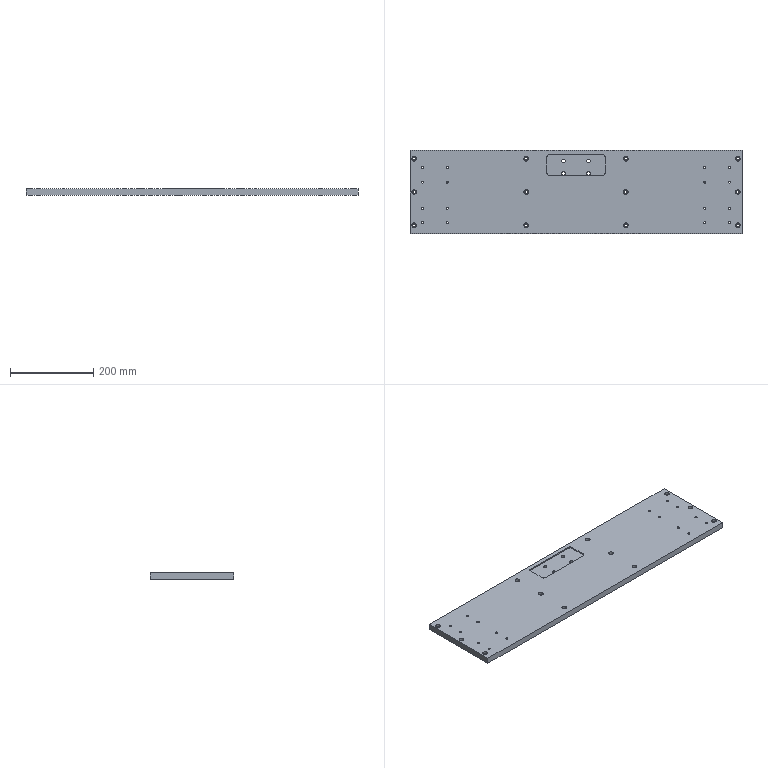Part | STEP file | 0244_222_Plate | 1 solid | 131 faces | box 800 x 200 x 15 mm | volume 2359509 mm3 | cylinder 100 | plane 23 | cone 8 | commonest cylinder face diameters 5 x40 6.6 x24 11 x24 8.5 x8 10 x4